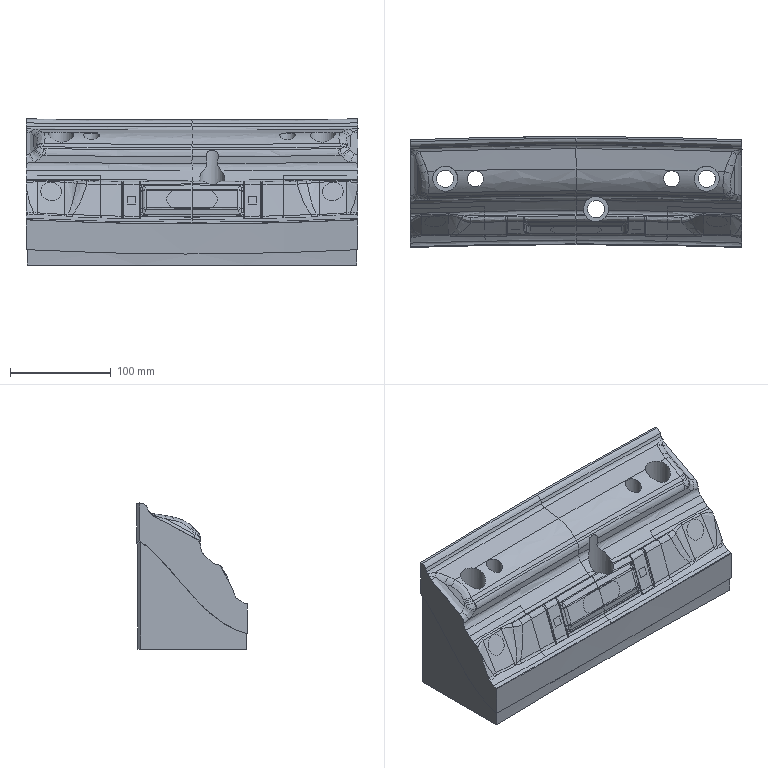Part | NX | features solid 2 | 1 solid | 267 faces | box 330.024 x 110.06 x 145.293 mm | volume 3410463 mm3 | spline 247 | plane 10 | cylinder 10 | commonest cylinder face diameters 25 x5 17 x3 16 x2